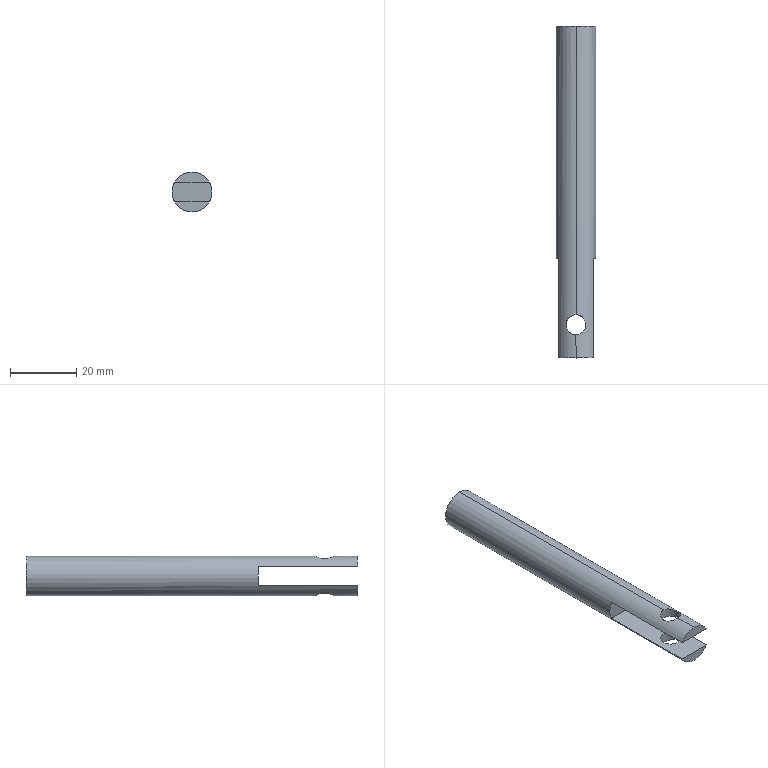Part | STEP file | Seat Rear Stay | 1 solid | 12 faces | box 12 x 100 x 12 mm | volume 9085 mm3 | cylinder 6 | plane 6 | commonest cylinder face diameters 6 x4 12 x2